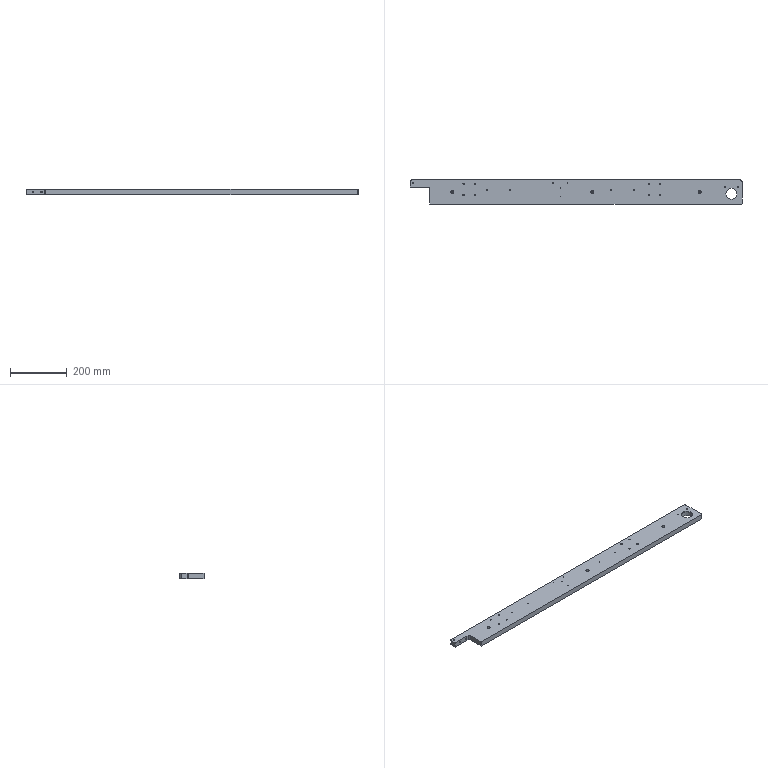Part | STEP file | 1 solid | 140 faces | box 1175 x 85 x 19 mm | volume 1780086 mm3 | cylinder 93 | cone 32 | plane 15 | commonest cylinder face diameters 3.3 x46 5 x16 11 x11 6 x6 2.5 x4 6.5 x4